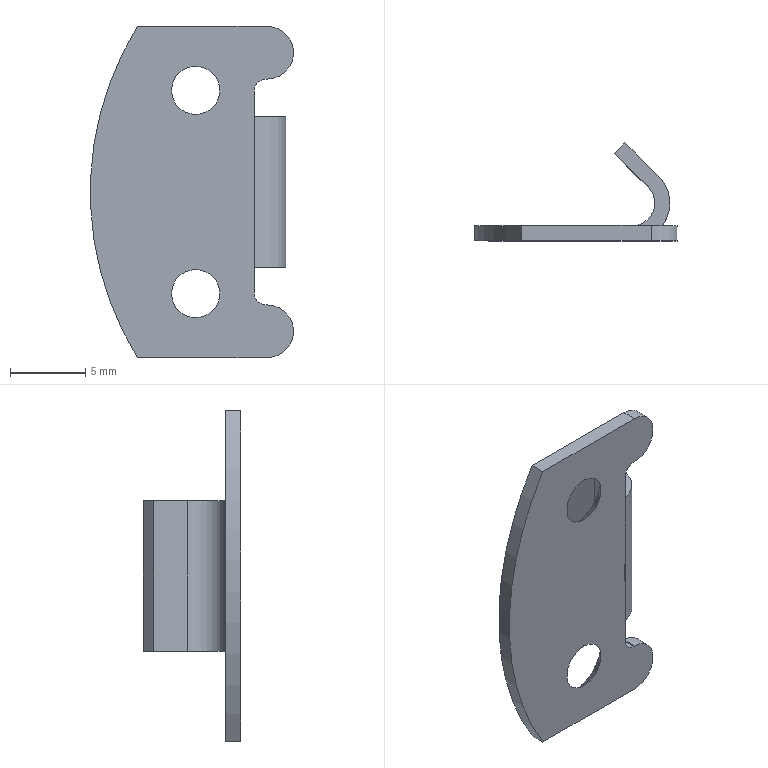Part | SolidWorks | features RefAxis 3, ICE 2, RevCut 2, 3DProfileFeature 1, Extrusion 1 | 1 solid | 23 faces | box 13.5 x 6.5 x 22 mm | volume 280.062 mm3 | plane 12 | cylinder 7 | cone 4 | commonest cylinder face diameters 1.6 x2 3.5 x2 3 x1 5 x1 41.74 x1
STEP:
#1=CARTESIAN_POINT('',(7.,0.,-8.35));
#2=VERTEX_POINT('',#1);
#3=CARTESIAN_POINT('',(7.,0.,-5.15));
#4=VERTEX_POINT('',#3);
#5=CARTESIAN_POINT('',(7.,0.,-6.75));
#6=DIRECTION('',(0.,1.,0.));
#7=DIRECTION('',(0.,0.,1.));
#8=AXIS2_PLACEMENT_3D('',#5,#6,#7);
#9=CIRCLE('',#8,1.6);
#10=EDGE_CURVE('',#2,#4,#9,.T.);
#11=ORIENTED_EDGE('',*,*,#10,.F.);
#12=CARTESIAN_POINT('',(7.,1.,-9.35));
#13=VERTEX_POINT('',#12);
#14=CARTESIAN_POINT('',(7.,0.,-8.35));
#15=DIRECTION('',(0.,0.7071,-0.7071));
#16=VECTOR('',#15,1000.);
#17=LINE('',#14,#16);
#18=EDGE_CURVE('',#2,#13,#17,.T.);
#19=ORIENTED_EDGE('',*,*,#18,.T.);
#20=CARTESIAN_POINT('',(7.,1.,-4.15));
#21=VERTEX_POINT('',#20);
#22=CARTESIAN_POINT('',(7.,1.,-6.75));
#23=DIRECTION('',(0.,1.,0.));
#24=DIRECTION('',(0.,0.,1.));
#25=AXIS2_PLACEMENT_3D('',#22,#23,#24);
#26=CIRCLE('',#25,2.6);
#27=EDGE_CURVE('',#13,#21,#26,.T.);
#28=ORIENTED_EDGE('',*,*,#27,.T.);
#29=CARTESIAN_POINT('',(7.,0.,-5.15));
#30=DIRECTION('',(0.,0.7071,0.7071));
#31=VECTOR('',#30,1000.);
#32=LINE('',#29,#31);
#33=EDGE_CURVE('',#4,#21,#32,.T.);
#34=ORIENTED_EDGE('',*,*,#33,.F.);
#35=EDGE_LOOP('',(#11,#19,#28,#34));
#36=FACE_OUTER_BOUND('',#35,.T.);
#37=CARTESIAN_POINT('',(7.,0.,-6.75));
#38=DIRECTION('',(0.,1.,0.));
#39=DIRECTION('',(0.,0.,1.));
#40=AXIS2_PLACEMENT_3D('',#37,#38,#39);
#41=CONICAL_SURFACE('',#40,1.6,0.7854);
#42=ADVANCED_FACE('',(#36),#41,.F.);
#43=CARTESIAN_POINT('',(7.,0.,5.15));
#44=VERTEX_POINT('',#43);
#45=CARTESIAN_POINT('',(7.,0.,8.35));
#46=VERTEX_POINT('',#45);
#47=CARTESIAN_POINT('',(7.,0.,6.75));
#48=DIRECTION('',(0.,1.,0.));
#49=DIRECTION('',(0.,0.,1.));
#50=AXIS2_PLACEMENT_3D('',#47,#48,#49);
#51=CIRCLE('',#50,1.6);
#52=EDGE_CURVE('',#44,#46,#51,.T.);
#53=ORIENTED_EDGE('',*,*,#52,.F.);
#54=CARTESIAN_POINT('',(7.,1.,4.15));
#55=VERTEX_POINT('',#54);
#56=CARTESIAN_POINT('',(7.,0.,5.15));
#57=DIRECTION('',(0.,0.7071,-0.7071));
#58=VECTOR('',#57,1000.);
#59=LINE('',#56,#58);
#60=EDGE_CURVE('',#44,#55,#59,.T.);
#61=ORIENTED_EDGE('',*,*,#60,.T.);
#62=CARTESIAN_POINT('',(7.,1.,9.35));
#63=VERTEX_POINT('',#62);
#64=CARTESIAN_POINT('',(7.,1.,6.75));
#65=DIRECTION('',(0.,1.,0.));
#66=DIRECTION('',(0.,0.,1.));
#67=AXIS2_PLACEMENT_3D('',#64,#65,#66);
#68=CIRCLE('',#67,2.6);
#69=EDGE_CURVE('',#55,#63,#68,.T.);
#70=ORIENTED_EDGE('',*,*,#69,.T.);
#71=CARTESIAN_POINT('',(7.,0.,8.35));
#72=DIRECTION('',(0.,0.7071,0.7071));
#73=VECTOR('',#72,1000.);
#74=LINE('',#71,#73);
#75=EDGE_CURVE('',#46,#63,#74,.T.);
#76=ORIENTED_EDGE('',*,*,#75,.F.);
#77=EDGE_LOOP('',(#53,#61,#70,#76));
#78=FACE_OUTER_BOUND('',#77,.T.);
#79=CARTESIAN_POINT('',(7.,0.,6.75));
#80=DIRECTION('',(0.,1.,0.));
#81=DIRECTION('',(0.,0.,1.));
#82=AXIS2_PLACEMENT_3D('',#79,#80,#81);
#83=CONICAL_SURFACE('',#82,1.6,0.7854);
#84=ADVANCED_FACE('',(#78),#83,.F.);
#85=CARTESIAN_POINT('',(7.,0.,6.75));
#86=DIRECTION('',(0.,1.,0.));
#87=DIRECTION('',(0.,0.,1.));
#88=AXIS2_PLACEMENT_3D('',#85,#86,#87);
#89=CIRCLE('',#88,1.6);
#90=EDGE_CURVE('',#46,#44,#89,.T.);
#91=ORIENTED_EDGE('',*,*,#90,.T.);
#92=ORIENTED_EDGE('',*,*,#52,.T.);
#93=EDGE_LOOP('',(#91,#92));
#94=FACE_BOUND('',#93,.T.);
#95=CARTESIAN_POINT('',(3.134,0.,11.));
#96=VERTEX_POINT('',#95);
#97=CARTESIAN_POINT('',(11.75,0.,11.));
#98=VERTEX_POINT('',#97);
#99=CARTESIAN_POINT('',(3.134,0.,11.));
#100=DIRECTION('',(1.,0.,0.));
#101=VECTOR('',#100,1000.);
#102=LINE('',#99,#101);
#103=EDGE_CURVE('',#96,#98,#102,.T.);
#104=ORIENTED_EDGE('',*,*,#103,.F.);
#105=CARTESIAN_POINT('',(3.134,0.,-11.));
#106=VERTEX_POINT('',#105);
#107=CARTESIAN_POINT('',(20.87,0.,0.));
#108=DIRECTION('',(0.,1.,0.));
#109=DIRECTION('',(0.,0.,1.));
#110=AXIS2_PLACEMENT_3D('',#107,#108,#109);
#111=CIRCLE('',#110,20.87);
#112=EDGE_CURVE('',#106,#96,#111,.T.);
#113=ORIENTED_EDGE('',*,*,#112,.F.);
#114=CARTESIAN_POINT('',(11.75,0.,-11.));
#115=VERTEX_POINT('',#114);
#116=CARTESIAN_POINT('',(11.75,0.,-11.));
#117=DIRECTION('',(-1.,0.,0.));
#118=VECTOR('',#117,1000.);
#119=LINE('',#116,#118);
#120=EDGE_CURVE('',#115,#106,#119,.T.);
#121=ORIENTED_EDGE('',*,*,#120,.F.);
#122=CARTESIAN_POINT('',(11.75,0.,-7.5));
#123=VERTEX_POINT('',#122);
#124=CARTESIAN_POINT('',(11.75,0.,-9.25));
#125=DIRECTION('',(0.,1.,0.));
#126=DIRECTION('',(0.,0.,1.));
#127=AXIS2_PLACEMENT_3D('',#124,#125,#126);
#128=CIRCLE('',#127,1.75);
#129=EDGE_CURVE('',#123,#115,#128,.T.);
#130=ORIENTED_EDGE('',*,*,#129,.F.);
#131=CARTESIAN_POINT('',(11.69,0.,-7.5));
#132=VERTEX_POINT('',#131);
#133=CARTESIAN_POINT('',(11.69,0.,-7.5));
#134=DIRECTION('',(1.,0.,0.));
#135=VECTOR('',#134,1000.);
#136=LINE('',#133,#135);
#137=EDGE_CURVE('',#132,#123,#136,.T.);
#138=ORIENTED_EDGE('',*,*,#137,.F.);
#139=CARTESIAN_POINT('',(10.89,0.,-6.7));
#140=VERTEX_POINT('',#139);
#141=CARTESIAN_POINT('',(11.69,0.,-6.7));
#142=DIRECTION('',(0.,-1.,0.));
#143=DIRECTION('',(0.,0.,-1.));
#144=AXIS2_PLACEMENT_3D('',#141,#142,#143);
#145=CIRCLE('',#144,0.8);
#146=EDGE_CURVE('',#140,#132,#145,.T.);
#147=ORIENTED_EDGE('',*,*,#146,.F.);
#148=CARTESIAN_POINT('',(10.89,0.,6.7));
#149=VERTEX_POINT('',#148);
#150=CARTESIAN_POINT('',(10.89,0.,6.7));
#151=DIRECTION('',(0.,0.,-1.));
#152=VECTOR('',#151,1000.);
#153=LINE('',#150,#152);
#154=EDGE_CURVE('',#149,#140,#153,.T.);
#155=ORIENTED_EDGE('',*,*,#154,.F.);
#156=CARTESIAN_POINT('',(11.69,0.,7.5));
#157=VERTEX_POINT('',#156);
#158=CARTESIAN_POINT('',(11.69,0.,6.7));
#159=DIRECTION('',(0.,-1.,0.));
#160=DIRECTION('',(0.,0.,-1.));
#161=AXIS2_PLACEMENT_3D('',#158,#159,#160);
#162=CIRCLE('',#161,0.8);
#163=EDGE_CURVE('',#157,#149,#162,.T.);
#164=ORIENTED_EDGE('',*,*,#163,.F.);
#165=CARTESIAN_POINT('',(11.75,0.,7.5));
#166=VERTEX_POINT('',#165);
#167=CARTESIAN_POINT('',(11.75,0.,7.5));
#168=DIRECTION('',(-1.,0.,0.));
#169=VECTOR('',#168,1000.);
#170=LINE('',#167,#169);
#171=EDGE_CURVE('',#166,#157,#170,.T.);
#172=ORIENTED_EDGE('',*,*,#171,.F.);
#173=CARTESIAN_POINT('',(11.75,0.,9.25));
#174=DIRECTION('',(0.,1.,0.));
#175=DIRECTION('',(0.,0.,1.));
#176=AXIS2_PLACEMENT_3D('',#173,#174,#175);
#177=CIRCLE('',#176,1.75);
#178=EDGE_CURVE('',#98,#166,#177,.T.);
#179=ORIENTED_EDGE('',*,*,#178,.F.);
#180=EDGE_LOOP('',(#104,#113,#121,#130,#138,#147,#155,#164,#172,#179));
#181=FACE_OUTER_BOUND('',#180,.T.);
#182=CARTESIAN_POINT('',(7.,0.,-6.75));
#183=DIRECTION('',(0.,1.,0.));
#184=DIRECTION('',(0.,0.,1.));
#185=AXIS2_PLACEMENT_3D('',#182,#183,#184);
#186=CIRCLE('',#185,1.6);
#187=EDGE_CURVE('',#4,#2,#186,.T.);
#188=ORIENTED_EDGE('',*,*,#187,.T.);
#189=ORIENTED_EDGE('',*,*,#10,.T.);
#190=EDGE_LOOP('',(#188,#189));
#191=FACE_BOUND('',#190,.T.);
#192=CARTESIAN_POINT('',(0.,0.,5.));
#193=DIRECTION('',(0.,1.,0.));
#194=DIRECTION('',(0.,0.,1.));
#195=AXIS2_PLACEMENT_3D('',#192,#193,#194);
#196=PLANE('',#195);
#197=ADVANCED_FACE('',(#94,#181,#191),#196,.F.);
#198=CARTESIAN_POINT('',(7.,1.,6.75));
#199=DIRECTION('',(0.,1.,0.));
#200=DIRECTION('',(0.,0.,1.));
#201=AXIS2_PLACEMENT_3D('',#198,#199,#200);
#202=CIRCLE('',#201,2.6);
#203=EDGE_CURVE('',#63,#55,#202,.T.);
#204=ORIENTED_EDGE('',*,*,#203,.F.);
#205=ORIENTED_EDGE('',*,*,#69,.F.);
#206=EDGE_LOOP('',(#204,#205));
#207=FACE_BOUND('',#206,.T.);
#208=CARTESIAN_POINT('',(3.134,1.,-11.));
#209=VERTEX_POINT('',#208);
#210=CARTESIAN_POINT('',(3.134,1.,11.));
#211=VERTEX_POINT('',#210);
#212=CARTESIAN_POINT('',(20.87,1.,0.));
#213=DIRECTION('',(0.,1.,0.));
#214=DIRECTION('',(0.,0.,1.));
#215=AXIS2_PLACEMENT_3D('',#212,#213,#214);
#216=CIRCLE('',#215,20.87);
#217=EDGE_CURVE('',#209,#211,#216,.T.);
#218=ORIENTED_EDGE('',*,*,#217,.T.);
#219=CARTESIAN_POINT('',(11.75,1.,11.));
#220=VERTEX_POINT('',#219);
#221=CARTESIAN_POINT('',(3.134,1.,11.));
#222=DIRECTION('',(1.,0.,0.));
#223=VECTOR('',#222,1000.);
#224=LINE('',#221,#223);
#225=EDGE_CURVE('',#211,#220,#224,.T.);
#226=ORIENTED_EDGE('',*,*,#225,.T.);
#227=CARTESIAN_POINT('',(11.75,1.,7.5));
#228=VERTEX_POINT('',#227);
#229=CARTESIAN_POINT('',(11.75,1.,9.25));
#230=DIRECTION('',(0.,1.,0.));
#231=DIRECTION('',(0.,0.,1.));
#232=AXIS2_PLACEMENT_3D('',#229,#230,#231);
#233=CIRCLE('',#232,1.75);
#234=EDGE_CURVE('',#220,#228,#233,.T.);
#235=ORIENTED_EDGE('',*,*,#234,.T.);
#236=CARTESIAN_POINT('',(11.69,1.,7.5));
#237=VERTEX_POINT('',#236);
#238=CARTESIAN_POINT('',(11.75,1.,7.5));
#239=DIRECTION('',(-1.,0.,0.));
#240=VECTOR('',#239,1000.);
#241=LINE('',#238,#240);
#242=EDGE_CURVE('',#228,#237,#241,.T.);
#243=ORIENTED_EDGE('',*,*,#242,.T.);
#244=CARTESIAN_POINT('',(10.89,1.,6.7));
#245=VERTEX_POINT('',#244);
#246=CARTESIAN_POINT('',(11.69,1.,6.7));
#247=DIRECTION('',(0.,-1.,0.));
#248=DIRECTION('',(0.,0.,-1.));
#249=AXIS2_PLACEMENT_3D('',#246,#247,#248);
#250=CIRCLE('',#249,0.8);
#251=EDGE_CURVE('',#237,#245,#250,.T.);
#252=ORIENTED_EDGE('',*,*,#251,.T.);
#253=CARTESIAN_POINT('',(10.89,1.,5.));
#254=VERTEX_POINT('',#253);
#255=CARTESIAN_POINT('',(10.89,1.,6.7));
#256=DIRECTION('',(0.,0.,-1.));
#257=VECTOR('',#256,1000.);
#258=LINE('',#255,#257);
#259=EDGE_CURVE('',#245,#254,#258,.T.);
#260=ORIENTED_EDGE('',*,*,#259,.T.);
#261=CARTESIAN_POINT('',(10.5,1.,5.));
#262=VERTEX_POINT('',#261);
#263=CARTESIAN_POINT('',(10.5,1.,5.));
#264=DIRECTION('',(-1.,0.,0.));
#265=VECTOR('',#264,1000.);
#266=LINE('',#263,#265);
#267=EDGE_CURVE('',#254,#262,#266,.T.);
#268=ORIENTED_EDGE('',*,*,#267,.T.);
#269=CARTESIAN_POINT('',(10.5,1.,-5.));
#270=VERTEX_POINT('',#269);
#271=CARTESIAN_POINT('',(10.5,1.,5.));
#272=DIRECTION('',(0.,0.,-1.));
#273=VECTOR('',#272,1000.);
#274=LINE('',#271,#273);
#275=EDGE_CURVE('',#262,#270,#274,.T.);
#276=ORIENTED_EDGE('',*,*,#275,.T.);
#277=CARTESIAN_POINT('',(10.89,1.,-5.));
#278=VERTEX_POINT('',#277);
#279=CARTESIAN_POINT('',(10.5,1.,-5.));
#280=DIRECTION('',(-1.,0.,0.));
#281=VECTOR('',#280,1000.);
#282=LINE('',#279,#281);
#283=EDGE_CURVE('',#278,#270,#282,.T.);
#284=ORIENTED_EDGE('',*,*,#283,.F.);
#285=CARTESIAN_POINT('',(10.89,1.,-6.7));
#286=VERTEX_POINT('',#285);
#287=CARTESIAN_POINT('',(10.89,1.,6.7));
#288=DIRECTION('',(0.,0.,-1.));
#289=VECTOR('',#288,1000.);
#290=LINE('',#287,#289);
#291=EDGE_CURVE('',#278,#286,#290,.T.);
#292=ORIENTED_EDGE('',*,*,#291,.T.);
#293=CARTESIAN_POINT('',(11.69,1.,-7.5));
#294=VERTEX_POINT('',#293);
#295=CARTESIAN_POINT('',(11.69,1.,-6.7));
#296=DIRECTION('',(0.,-1.,0.));
#297=DIRECTION('',(0.,0.,-1.));
#298=AXIS2_PLACEMENT_3D('',#295,#296,#297);
#299=CIRCLE('',#298,0.8);
#300=EDGE_CURVE('',#286,#294,#299,.T.);
#301=ORIENTED_EDGE('',*,*,#300,.T.);
#302=CARTESIAN_POINT('',(11.75,1.,-7.5));
#303=VERTEX_POINT('',#302);
#304=CARTESIAN_POINT('',(11.69,1.,-7.5));
#305=DIRECTION('',(1.,0.,0.));
#306=VECTOR('',#305,1000.);
#307=LINE('',#304,#306);
#308=EDGE_CURVE('',#294,#303,#307,.T.);
#309=ORIENTED_EDGE('',*,*,#308,.T.);
#310=CARTESIAN_POINT('',(11.75,1.,-11.));
#311=VERTEX_POINT('',#310);
#312=CARTESIAN_POINT('',(11.75,1.,-9.25));
#313=DIRECTION('',(0.,1.,0.));
#314=DIRECTION('',(0.,0.,1.));
#315=AXIS2_PLACEMENT_3D('',#312,#313,#314);
#316=CIRCLE('',#315,1.75);
#317=EDGE_CURVE('',#303,#311,#316,.T.);
#318=ORIENTED_EDGE('',*,*,#317,.T.);
#319=CARTESIAN_POINT('',(11.75,1.,-11.));
#320=DIRECTION('',(-1.,0.,0.));
#321=VECTOR('',#320,1000.);
#322=LINE('',#319,#321);
#323=EDGE_CURVE('',#311,#209,#322,.T.);
#324=ORIENTED_EDGE('',*,*,#323,.T.);
#325=EDGE_LOOP('',(#218,#226,#235,#243,#252,#260,#268,#276,#284,#292,#301,#309,#318,#324));
#326=FACE_OUTER_BOUND('',#325,.T.);
#327=CARTESIAN_POINT('',(7.,1.,-6.75));
#328=DIRECTION('',(0.,1.,0.));
#329=DIRECTION('',(0.,0.,1.));
#330=AXIS2_PLACEMENT_3D('',#327,#328,#329);
#331=CIRCLE('',#330,2.6);
#332=EDGE_CURVE('',#21,#13,#331,.T.);
#333=ORIENTED_EDGE('',*,*,#332,.F.);
#334=ORIENTED_EDGE('',*,*,#27,.F.);
#335=EDGE_LOOP('',(#333,#334));
#336=FACE_BOUND('',#335,.T.);
#337=CARTESIAN_POINT('',(10.5,1.,5.));
#338=DIRECTION('',(0.,-1.,0.));
#339=DIRECTION('',(0.,0.,-1.));
#340=AXIS2_PLACEMENT_3D('',#337,#338,#339);
#341=PLANE('',#340);
#342=ADVANCED_FACE('',(#207,#326,#336),#341,.F.);
#343=CARTESIAN_POINT('',(10.89,0.03061,-5.));
#344=VERTEX_POINT('',#343);
#345=CARTESIAN_POINT('',(10.89,0.03061,5.));
#346=VERTEX_POINT('',#345);
#347=CARTESIAN_POINT('',(10.89,0.03061,5.));
#348=DIRECTION('',(0.,0.,1.));
#349=VECTOR('',#348,1000.);
#350=LINE('',#347,#349);
#351=EDGE_CURVE('',#344,#346,#350,.T.);
#352=ORIENTED_EDGE('',*,*,#351,.F.);
#353=CARTESIAN_POINT('',(12.254,4.282,-5.));
#354=VERTEX_POINT('',#353);
#355=CARTESIAN_POINT('',(10.5,2.5,-5.));
#356=DIRECTION('',(0.,0.,1.));
#357=DIRECTION('',(1.,0.,0.));
#358=AXIS2_PLACEMENT_3D('',#355,#356,#357);
#359=CIRCLE('',#358,2.5);
#360=EDGE_CURVE('',#344,#354,#359,.T.);
#361=ORIENTED_EDGE('',*,*,#360,.T.);
#362=CARTESIAN_POINT('',(12.254,4.282,5.));
#363=VERTEX_POINT('',#362);
#364=CARTESIAN_POINT('',(12.254,4.282,5.));
#365=DIRECTION('',(0.,0.,-1.));
#366=VECTOR('',#365,1000.);
#367=LINE('',#364,#366);
#368=EDGE_CURVE('',#363,#354,#367,.T.);
#369=ORIENTED_EDGE('',*,*,#368,.F.);
#370=CARTESIAN_POINT('',(10.5,2.5,5.));
#371=DIRECTION('',(0.,0.,1.));
#372=DIRECTION('',(1.,0.,0.));
#373=AXIS2_PLACEMENT_3D('',#370,#371,#372);
#374=CIRCLE('',#373,2.5);
#375=EDGE_CURVE('',#346,#363,#374,.T.);
#376=ORIENTED_EDGE('',*,*,#375,.F.);
#377=EDGE_LOOP('',(#352,#361,#369,#376));
#378=FACE_OUTER_BOUND('',#377,.T.);
#379=CARTESIAN_POINT('',(10.5,2.5,5.));
#380=DIRECTION('',(0.,0.,-1.));
#381=DIRECTION('',(-1.,0.,0.));
#382=AXIS2_PLACEMENT_3D('',#379,#380,#381);
#383=CYLINDRICAL_SURFACE('',#382,2.5);
#384=ADVANCED_FACE('',(#378),#383,.T.);
#385=ORIENTED_EDGE('',*,*,#267,.F.);
#386=CARTESIAN_POINT('',(10.89,2.5,5.));
#387=DIRECTION('',(0.,-1.,0.));
#388=VECTOR('',#387,1000.);
#389=LINE('',#386,#388);
#390=EDGE_CURVE('',#254,#346,#389,.T.);
#391=ORIENTED_EDGE('',*,*,#390,.T.);
#392=ORIENTED_EDGE('',*,*,#375,.T.);
#393=CARTESIAN_POINT('',(10.,6.5,5.));
#394=VERTEX_POINT('',#393);
#395=CARTESIAN_POINT('',(12.254,4.282,5.));
#396=DIRECTION('',(-0.7127,0.7015,0.));
#397=VECTOR('',#396,1000.);
#398=LINE('',#395,#397);
#399=EDGE_CURVE('',#363,#394,#398,.T.);
#400=ORIENTED_EDGE('',*,*,#399,.T.);
#401=CARTESIAN_POINT('',(9.299,5.787,5.));
#402=VERTEX_POINT('',#401);
#403=CARTESIAN_POINT('',(10.,6.5,5.));
#404=DIRECTION('',(-0.7015,-0.7127,0.));
#405=VECTOR('',#404,1000.);
#406=LINE('',#403,#405);
#407=EDGE_CURVE('',#394,#402,#406,.T.);
#408=ORIENTED_EDGE('',*,*,#407,.T.);
#409=CARTESIAN_POINT('',(11.552,3.569,5.));
#410=VERTEX_POINT('',#409);
#411=CARTESIAN_POINT('',(9.299,5.787,5.));
#412=DIRECTION('',(0.7127,-0.7015,0.));
#413=VECTOR('',#412,1000.);
#414=LINE('',#411,#413);
#415=EDGE_CURVE('',#402,#410,#414,.T.);
#416=ORIENTED_EDGE('',*,*,#415,.T.);
#417=CARTESIAN_POINT('',(10.5,2.5,5.));
#418=DIRECTION('',(0.,0.,-1.));
#419=DIRECTION('',(-1.,0.,0.));
#420=AXIS2_PLACEMENT_3D('',#417,#418,#419);
#421=CIRCLE('',#420,1.5);
#422=EDGE_CURVE('',#410,#262,#421,.T.);
#423=ORIENTED_EDGE('',*,*,#422,.T.);
#424=EDGE_LOOP('',(#385,#391,#392,#400,#408,#416,#423));
#425=FACE_OUTER_BOUND('',#424,.T.);
#426=CARTESIAN_POINT('',(10.5,2.5,5.));
#427=DIRECTION('',(0.,0.,1.));
#428=DIRECTION('',(1.,0.,0.));
#429=AXIS2_PLACEMENT_3D('',#426,#427,#428);
#430=PLANE('',#429);
#431=ADVANCED_FACE('',(#425),#430,.T.);
#432=CARTESIAN_POINT('',(10.89,2.5,-5.));
#433=DIRECTION('',(0.,-1.,0.));
#434=VECTOR('',#433,1000.);
#435=LINE('',#432,#434);
#436=EDGE_CURVE('',#278,#344,#435,.T.);
#437=ORIENTED_EDGE('',*,*,#436,.F.);
#438=ORIENTED_EDGE('',*,*,#283,.T.);
#439=CARTESIAN_POINT('',(11.552,3.569,-5.));
#440=VERTEX_POINT('',#439);
#441=CARTESIAN_POINT('',(10.5,2.5,-5.));
#442=DIRECTION('',(0.,0.,-1.));
#443=DIRECTION('',(-1.,0.,0.));
#444=AXIS2_PLACEMENT_3D('',#441,#442,#443);
#445=CIRCLE('',#444,1.5);
#446=EDGE_CURVE('',#440,#270,#445,.T.);
#447=ORIENTED_EDGE('',*,*,#446,.F.);
#448=CARTESIAN_POINT('',(9.299,5.787,-5.));
#449=VERTEX_POINT('',#448);
#450=CARTESIAN_POINT('',(9.299,5.787,-5.));
#451=DIRECTION('',(0.7127,-0.7015,0.));
#452=VECTOR('',#451,1000.);
#453=LINE('',#450,#452);
#454=EDGE_CURVE('',#449,#440,#453,.T.);
#455=ORIENTED_EDGE('',*,*,#454,.F.);
#456=CARTESIAN_POINT('',(10.,6.5,-5.));
#457=VERTEX_POINT('',#456);
#458=CARTESIAN_POINT('',(10.,6.5,-5.));
#459=DIRECTION('',(-0.7015,-0.7127,0.));
#460=VECTOR('',#459,1000.);
#461=LINE('',#458,#460);
#462=EDGE_CURVE('',#457,#449,#461,.T.);
#463=ORIENTED_EDGE('',*,*,#462,.F.);
#464=CARTESIAN_POINT('',(12.254,4.282,-5.));
#465=DIRECTION('',(-0.7127,0.7015,0.));
#466=VECTOR('',#465,1000.);
#467=LINE('',#464,#466);
#468=EDGE_CURVE('',#354,#457,#467,.T.);
#469=ORIENTED_EDGE('',*,*,#468,.F.);
#470=ORIENTED_EDGE('',*,*,#360,.F.);
#471=EDGE_LOOP('',(#437,#438,#447,#455,#463,#469,#470));
#472=FACE_OUTER_BOUND('',#471,.T.);
#473=CARTESIAN_POINT('',(10.5,2.5,-5.));
#474=DIRECTION('',(0.,0.,1.));
#475=DIRECTION('',(1.,0.,0.));
#476=AXIS2_PLACEMENT_3D('',#473,#474,#475);
#477=PLANE('',#476);
#478=ADVANCED_FACE('',(#472),#477,.F.);
#479=ORIENTED_EDGE('',*,*,#368,.T.);
#480=ORIENTED_EDGE('',*,*,#468,.T.);
#481=CARTESIAN_POINT('',(10.,6.5,5.));
#482=DIRECTION('',(0.,0.,-1.));
#483=VECTOR('',#482,1000.);
#484=LINE('',#481,#483);
#485=EDGE_CURVE('',#394,#457,#484,.T.);
#486=ORIENTED_EDGE('',*,*,#485,.F.);
#487=ORIENTED_EDGE('',*,*,#399,.F.);
#488=EDGE_LOOP('',(#479,#480,#486,#487));
#489=FACE_OUTER_BOUND('',#488,.T.);
#490=CARTESIAN_POINT('',(12.254,4.282,5.));
#491=DIRECTION('',(-0.7015,-0.7127,0.));
#492=DIRECTION('',(0.7127,-0.7015,0.));
#493=AXIS2_PLACEMENT_3D('',#490,#491,#492);
#494=PLANE('',#493);
#495=ADVANCED_FACE('',(#489),#494,.F.);
#496=ORIENTED_EDGE('',*,*,#485,.T.);
#497=ORIENTED_EDGE('',*,*,#462,.T.);
#498=CARTESIAN_POINT('',(9.299,5.787,5.));
#499=DIRECTION('',(0.,0.,-1.));
#500=VECTOR('',#499,1000.);
#501=LINE('',#498,#500);
#502=EDGE_CURVE('',#402,#449,#501,.T.);
#503=ORIENTED_EDGE('',*,*,#502,.F.);
#504=ORIENTED_EDGE('',*,*,#407,.F.);
#505=EDGE_LOOP('',(#496,#497,#503,#504));
#506=FACE_OUTER_BOUND('',#505,.T.);
#507=CARTESIAN_POINT('',(10.,6.5,5.));
#508=DIRECTION('',(0.7127,-0.7015,0.));
#509=DIRECTION('',(0.7015,0.7127,0.));
#510=AXIS2_PLACEMENT_3D('',#507,#508,#509);
#511=PLANE('',#510);
#512=ADVANCED_FACE('',(#506),#511,.F.);
#513=ORIENTED_EDGE('',*,*,#502,.T.);
#514=ORIENTED_EDGE('',*,*,#454,.T.);
#515=CARTESIAN_POINT('',(11.552,3.569,5.));
#516=DIRECTION('',(0.,0.,-1.));
#517=VECTOR('',#516,1000.);
#518=LINE('',#515,#517);
#519=EDGE_CURVE('',#410,#440,#518,.T.);
#520=ORIENTED_EDGE('',*,*,#519,.F.);
#521=ORIENTED_EDGE('',*,*,#415,.F.);
#522=EDGE_LOOP('',(#513,#514,#520,#521));
#523=FACE_OUTER_BOUND('',#522,.T.);
#524=CARTESIAN_POINT('',(9.299,5.787,5.));
#525=DIRECTION('',(0.7015,0.7127,0.));
#526=DIRECTION('',(-0.7127,0.7015,0.));
#527=AXIS2_PLACEMENT_3D('',#524,#525,#526);
#528=PLANE('',#527);
#529=ADVANCED_FACE('',(#523),#528,.F.);
#530=ORIENTED_EDGE('',*,*,#519,.T.);
#531=ORIENTED_EDGE('',*,*,#446,.T.);
#532=ORIENTED_EDGE('',*,*,#275,.F.);
#533=ORIENTED_EDGE('',*,*,#422,.F.);
#534=EDGE_LOOP('',(#530,#531,#532,#533));
#535=FACE_OUTER_BOUND('',#534,.T.);
#536=CARTESIAN_POINT('',(10.5,2.5,5.));
#537=DIRECTION('',(0.,0.,-1.));
#538=DIRECTION('',(-1.,0.,0.));
#539=AXIS2_PLACEMENT_3D('',#536,#537,#538);
#540=CYLINDRICAL_SURFACE('',#539,1.5);
#541=ADVANCED_FACE('',(#535),#540,.F.);
#542=ORIENTED_EDGE('',*,*,#112,.T.);
#543=CARTESIAN_POINT('',(3.134,1.,11.));
#544=DIRECTION('',(0.,-1.,0.));
#545=VECTOR('',#544,1000.);
#546=LINE('',#543,#545);
#547=EDGE_CURVE('',#211,#96,#546,.T.);
#548=ORIENTED_EDGE('',*,*,#547,.F.);
#549=ORIENTED_EDGE('',*,*,#217,.F.);
#550=CARTESIAN_POINT('',(3.134,1.,-11.));
#551=DIRECTION('',(0.,-1.,0.));
#552=VECTOR('',#551,1000.);
#553=LINE('',#550,#552);
#554=EDGE_CURVE('',#209,#106,#553,.T.);
#555=ORIENTED_EDGE('',*,*,#554,.T.);
#556=EDGE_LOOP('',(#542,#548,#549,#555));
#557=FACE_OUTER_BOUND('',#556,.T.);
#558=CARTESIAN_POINT('',(20.87,1.,0.));
#559=DIRECTION('',(0.,-1.,0.));
#560=DIRECTION('',(0.,0.,-1.));
#561=AXIS2_PLACEMENT_3D('',#558,#559,#560);
#562=CYLINDRICAL_SURFACE('',#561,20.87);
#563=ADVANCED_FACE('',(#557),#562,.T.);
#564=ORIENTED_EDGE('',*,*,#103,.T.);
#565=CARTESIAN_POINT('',(11.75,1.,11.));
#566=DIRECTION('',(0.,-1.,0.));
#567=VECTOR('',#566,1000.);
#568=LINE('',#565,#567);
#569=EDGE_CURVE('',#220,#98,#568,.T.);
#570=ORIENTED_EDGE('',*,*,#569,.F.);
#571=ORIENTED_EDGE('',*,*,#225,.F.);
#572=ORIENTED_EDGE('',*,*,#547,.T.);
#573=EDGE_LOOP('',(#564,#570,#571,#572));
#574=FACE_OUTER_BOUND('',#573,.T.);
#575=CARTESIAN_POINT('',(3.134,1.,11.));
#576=DIRECTION('',(0.,0.,-1.));
#577=DIRECTION('',(-1.,0.,0.));
#578=AXIS2_PLACEMENT_3D('',#575,#576,#577);
#579=PLANE('',#578);
#580=ADVANCED_FACE('',(#574),#579,.F.);
#581=ORIENTED_EDGE('',*,*,#178,.T.);
#582=CARTESIAN_POINT('',(11.75,1.,7.5));
#583=DIRECTION('',(0.,-1.,0.));
#584=VECTOR('',#583,1000.);
#585=LINE('',#582,#584);
#586=EDGE_CURVE('',#228,#166,#585,.T.);
#587=ORIENTED_EDGE('',*,*,#586,.F.);
#588=ORIENTED_EDGE('',*,*,#234,.F.);
#589=ORIENTED_EDGE('',*,*,#569,.T.);
#590=EDGE_LOOP('',(#581,#587,#588,#589));
#591=FACE_OUTER_BOUND('',#590,.T.);
#592=CARTESIAN_POINT('',(11.75,1.,9.25));
#593=DIRECTION('',(0.,-1.,0.));
#594=DIRECTION('',(0.,0.,-1.));
#595=AXIS2_PLACEMENT_3D('',#592,#593,#594);
#596=CYLINDRICAL_SURFACE('',#595,1.75);
#597=ADVANCED_FACE('',(#591),#596,.T.);
#598=ORIENTED_EDGE('',*,*,#171,.T.);
#599=CARTESIAN_POINT('',(11.69,1.,7.5));
#600=DIRECTION('',(0.,-1.,0.));
#601=VECTOR('',#600,1000.);
#602=LINE('',#599,#601);
#603=EDGE_CURVE('',#237,#157,#602,.T.);
#604=ORIENTED_EDGE('',*,*,#603,.F.);
#605=ORIENTED_EDGE('',*,*,#242,.F.);
#606=ORIENTED_EDGE('',*,*,#586,.T.);
#607=EDGE_LOOP('',(#598,#604,#605,#606));
#608=FACE_OUTER_BOUND('',#607,.T.);
#609=CARTESIAN_POINT('',(11.75,1.,7.5));
#610=DIRECTION('',(0.,0.,1.));
#611=DIRECTION('',(1.,0.,0.));
#612=AXIS2_PLACEMENT_3D('',#609,#610,#611);
#613=PLANE('',#612);
#614=ADVANCED_FACE('',(#608),#613,.F.);
#615=ORIENTED_EDGE('',*,*,#163,.T.);
#616=CARTESIAN_POINT('',(10.89,1.,6.7));
#617=DIRECTION('',(0.,-1.,0.));
#618=VECTOR('',#617,1000.);
#619=LINE('',#616,#618);
#620=EDGE_CURVE('',#245,#149,#619,.T.);
#621=ORIENTED_EDGE('',*,*,#620,.F.);
#622=ORIENTED_EDGE('',*,*,#251,.F.);
#623=ORIENTED_EDGE('',*,*,#603,.T.);
#624=EDGE_LOOP('',(#615,#621,#622,#623));
#625=FACE_OUTER_BOUND('',#624,.T.);
#626=CARTESIAN_POINT('',(11.69,1.,6.7));
#627=DIRECTION('',(0.,-1.,0.));
#628=DIRECTION('',(0.,0.,-1.));
#629=AXIS2_PLACEMENT_3D('',#626,#627,#628);
#630=CYLINDRICAL_SURFACE('',#629,0.8);
#631=ADVANCED_FACE('',(#625),#630,.F.);
#632=ORIENTED_EDGE('',*,*,#390,.F.);
#633=ORIENTED_EDGE('',*,*,#259,.F.);
#634=ORIENTED_EDGE('',*,*,#620,.T.);
#635=ORIENTED_EDGE('',*,*,#154,.T.);
#636=CARTESIAN_POINT('',(10.89,1.,-6.7));
#637=DIRECTION('',(0.,-1.,0.));
#638=VECTOR('',#637,1000.);
#639=LINE('',#636,#638);
#640=EDGE_CURVE('',#286,#140,#639,.T.);
#641=ORIENTED_EDGE('',*,*,#640,.F.);
#642=ORIENTED_EDGE('',*,*,#291,.F.);
#643=ORIENTED_EDGE('',*,*,#436,.T.);
#644=ORIENTED_EDGE('',*,*,#351,.T.);
#645=EDGE_LOOP('',(#632,#633,#634,#635,#641,#642,#643,#644));
#646=FACE_OUTER_BOUND('',#645,.T.);
#647=CARTESIAN_POINT('',(10.89,1.,6.7));
#648=DIRECTION('',(-1.,0.,0.));
#649=DIRECTION('',(0.,0.,1.));
#650=AXIS2_PLACEMENT_3D('',#647,#648,#649);
#651=PLANE('',#650);
#652=ADVANCED_FACE('',(#646),#651,.F.);
#653=ORIENTED_EDGE('',*,*,#146,.T.);
#654=CARTESIAN_POINT('',(11.69,1.,-7.5));
#655=DIRECTION('',(0.,-1.,0.));
#656=VECTOR('',#655,1000.);
#657=LINE('',#654,#656);
#658=EDGE_CURVE('',#294,#132,#657,.T.);
#659=ORIENTED_EDGE('',*,*,#658,.F.);
#660=ORIENTED_EDGE('',*,*,#300,.F.);
#661=ORIENTED_EDGE('',*,*,#640,.T.);
#662=EDGE_LOOP('',(#653,#659,#660,#661));
#663=FACE_OUTER_BOUND('',#662,.T.);
#664=CARTESIAN_POINT('',(11.69,1.,-6.7));
#665=DIRECTION('',(0.,-1.,0.));
#666=DIRECTION('',(0.,0.,-1.));
#667=AXIS2_PLACEMENT_3D('',#664,#665,#666);
#668=CYLINDRICAL_SURFACE('',#667,0.8);
#669=ADVANCED_FACE('',(#663),#668,.F.);
#670=ORIENTED_EDGE('',*,*,#137,.T.);
#671=CARTESIAN_POINT('',(11.75,1.,-7.5));
#672=DIRECTION('',(0.,-1.,0.));
#673=VECTOR('',#672,1000.);
#674=LINE('',#671,#673);
#675=EDGE_CURVE('',#303,#123,#674,.T.);
#676=ORIENTED_EDGE('',*,*,#675,.F.);
#677=ORIENTED_EDGE('',*,*,#308,.F.);
#678=ORIENTED_EDGE('',*,*,#658,.T.);
#679=EDGE_LOOP('',(#670,#676,#677,#678));
#680=FACE_OUTER_BOUND('',#679,.T.);
#681=CARTESIAN_POINT('',(11.69,1.,-7.5));
#682=DIRECTION('',(0.,0.,-1.));
#683=DIRECTION('',(-1.,0.,0.));
#684=AXIS2_PLACEMENT_3D('',#681,#682,#683);
#685=PLANE('',#684);
#686=ADVANCED_FACE('',(#680),#685,.F.);
#687=ORIENTED_EDGE('',*,*,#129,.T.);
#688=CARTESIAN_POINT('',(11.75,1.,-11.));
#689=DIRECTION('',(0.,-1.,0.));
#690=VECTOR('',#689,1000.);
#691=LINE('',#688,#690);
#692=EDGE_CURVE('',#311,#115,#691,.T.);
#693=ORIENTED_EDGE('',*,*,#692,.F.);
#694=ORIENTED_EDGE('',*,*,#317,.F.);
#695=ORIENTED_EDGE('',*,*,#675,.T.);
#696=EDGE_LOOP('',(#687,#693,#694,#695));
#697=FACE_OUTER_BOUND('',#696,.T.);
#698=CARTESIAN_POINT('',(11.75,1.,-9.25));
#699=DIRECTION('',(0.,-1.,0.));
#700=DIRECTION('',(0.,0.,-1.));
#701=AXIS2_PLACEMENT_3D('',#698,#699,#700);
#702=CYLINDRICAL_SURFACE('',#701,1.75);
#703=ADVANCED_FACE('',(#697),#702,.T.);
#704=ORIENTED_EDGE('',*,*,#120,.T.);
#705=ORIENTED_EDGE('',*,*,#554,.F.);
#706=ORIENTED_EDGE('',*,*,#323,.F.);
#707=ORIENTED_EDGE('',*,*,#692,.T.);
#708=EDGE_LOOP('',(#704,#705,#706,#707));
#709=FACE_OUTER_BOUND('',#708,.T.);
#710=CARTESIAN_POINT('',(11.75,1.,-11.));
#711=DIRECTION('',(0.,0.,1.));
#712=DIRECTION('',(1.,0.,0.));
#713=AXIS2_PLACEMENT_3D('',#710,#711,#712);
#714=PLANE('',#713);
#715=ADVANCED_FACE('',(#709),#714,.F.);
#716=ORIENTED_EDGE('',*,*,#60,.F.);
#717=ORIENTED_EDGE('',*,*,#90,.F.);
#718=ORIENTED_EDGE('',*,*,#75,.T.);
#719=ORIENTED_EDGE('',*,*,#203,.T.);
#720=EDGE_LOOP('',(#716,#717,#718,#719));
#721=FACE_OUTER_BOUND('',#720,.T.);
#722=CARTESIAN_POINT('',(7.,0.,6.75));
#723=DIRECTION('',(0.,1.,0.));
#724=DIRECTION('',(0.,0.,1.));
#725=AXIS2_PLACEMENT_3D('',#722,#723,#724);
#726=CONICAL_SURFACE('',#725,1.6,0.7854);
#727=ADVANCED_FACE('',(#721),#726,.F.);
#728=ORIENTED_EDGE('',*,*,#18,.F.);
#729=ORIENTED_EDGE('',*,*,#187,.F.);
#730=ORIENTED_EDGE('',*,*,#33,.T.);
#731=ORIENTED_EDGE('',*,*,#332,.T.);
#732=EDGE_LOOP('',(#728,#729,#730,#731));
#733=FACE_OUTER_BOUND('',#732,.T.);
#734=CARTESIAN_POINT('',(7.,0.,-6.75));
#735=DIRECTION('',(0.,1.,0.));
#736=DIRECTION('',(0.,0.,1.));
#737=AXIS2_PLACEMENT_3D('',#734,#735,#736);
#738=CONICAL_SURFACE('',#737,1.6,0.7854);
#739=ADVANCED_FACE('',(#733),#738,.F.);
#740=CLOSED_SHELL('',(#42,#84,#197,#342,#384,#431,#478,#495,#512,#529,#541,#563,#580,#597,#614,#631,#652,#669,#686,#703,#715,#727,#739));
#741=MANIFOLD_SOLID_BREP('',#740);
#742=CARTESIAN_POINT('',(0.,0.,0.));
#743=DIRECTION('',(0.,0.,1.));
#744=DIRECTION('',(1.,0.,0.));
#745=AXIS2_PLACEMENT_3D('',#742,#743,#744);
#746=(LENGTH_UNIT()NAMED_UNIT(*)SI_UNIT(.MILLI.,.METRE.));
#747=UNCERTAINTY_MEASURE_WITH_UNIT(LENGTH_MEASURE(0.00001),#746,'','');
#748=(NAMED_UNIT(*)PLANE_ANGLE_UNIT()SI_UNIT($,.RADIAN.));
#749=(NAMED_UNIT(*)SI_UNIT($,.STERADIAN.)SOLID_ANGLE_UNIT());
#750=(GEOMETRIC_REPRESENTATION_CONTEXT(3)GLOBAL_UNCERTAINTY_ASSIGNED_CONTEXT((#747))GLOBAL_UNIT_ASSIGNED_CONTEXT((#746,#748,#749))REPRESENTATION_CONTEXT('',''));
#751=ADVANCED_BREP_SHAPE_REPRESENTATION('',(#741,#745),#750);